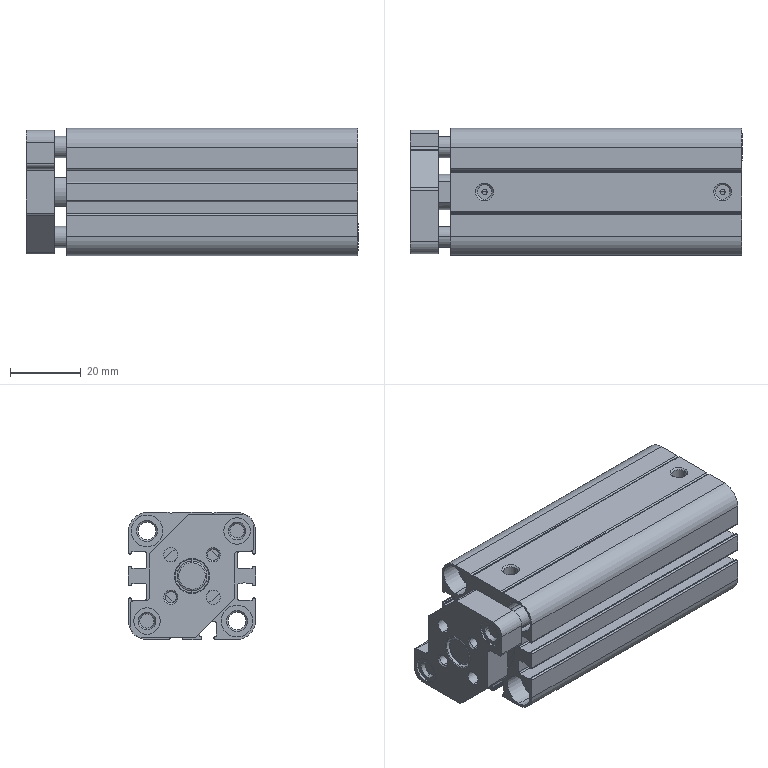Part | SolidWorks | features BaseBody 2 | 2 solids | 308 faces | box 94 x 36 x 36 mm | volume 78823 mm3 | cylinder 147 | plane 111 | cone 42 | spline 8 | commonest cylinder face diameters 0.4 x29 0.8 x24 9 x12 2 x8 4.917 x8 6 x8